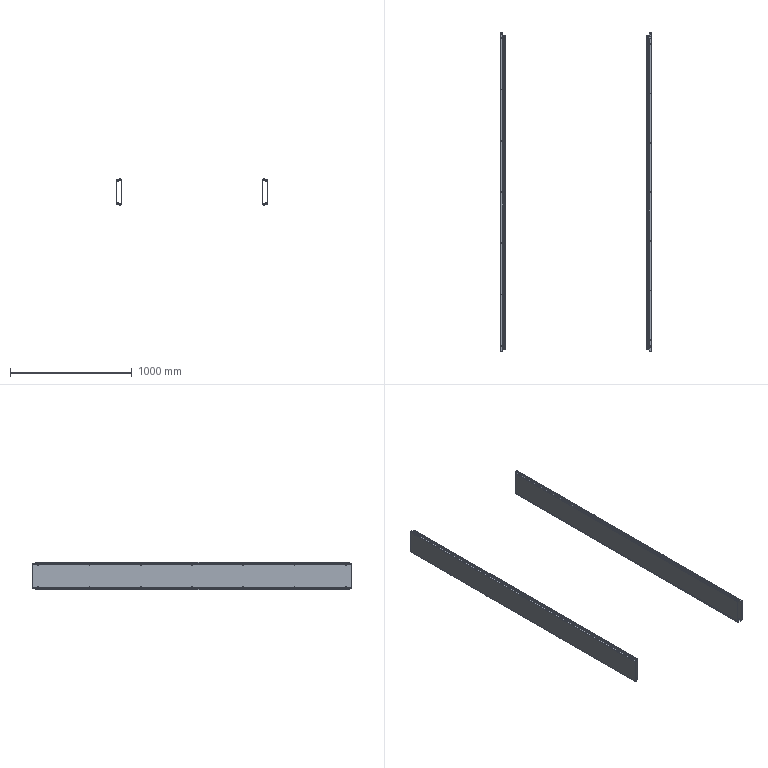Part | 36 solids | 953 faces | box 1240 x 2616 x 227 mm | volume 4657700 mm3 | plane 562 | cylinder 391 | commonest cylinder face diameters 6 x56 6.2 x56 8 x56 12 x56 6.4 x48 0.6 x40